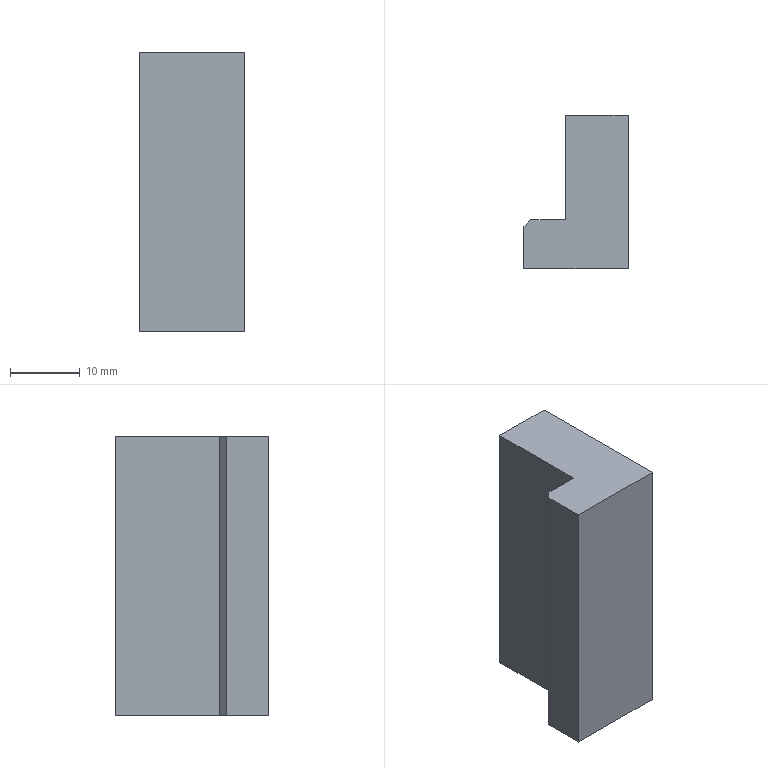Part | STEP file | ASND-0110-Body 1-30 | 1 solid | 9 faces | box 15 x 22 x 40 mm | volume 9580 mm3 | plane 9
STEP:
#1=CARTESIAN_POINT('',(0.,0.,0.));
#2=DIRECTION('',(0.,0.,1.));
#3=DIRECTION('',(1.,0.,0.));
#4=AXIS2_PLACEMENT_3D('',#1,#2,#3);
#5=CARTESIAN_POINT('',(1.,7.,14.));
#6=VERTEX_POINT('',#5);
#7=CARTESIAN_POINT('',(0.,6.,14.));
#8=VERTEX_POINT('',#7);
#9=CARTESIAN_POINT('',(3.,9.,14.));
#10=DIRECTION('',(-0.7071,-0.7071,0.));
#11=VECTOR('',#10,1.);
#12=LINE('',#9,#11);
#13=CARTESIAN_POINT('',(0.5,6.5,27.));
#14=DIRECTION('',(-0.7071,0.7071,0.));
#15=DIRECTION('',(0.5774,0.5774,0.5774));
#16=AXIS2_PLACEMENT_3D('',#13,#14,#15);
#17=PLANE('',#16);
#18=CARTESIAN_POINT('',(-4.619,12.656));
#19=DIRECTION('',(-0.8165,-0.5774));
#20=VECTOR('',#19,1.);
#21=LINE('',#18,#20);
#22=(GEOMETRIC_REPRESENTATION_CONTEXT(2)PARAMETRIC_REPRESENTATION_CONTEXT()REPRESENTATION_CONTEXT('',''));
#23=DEFINITIONAL_REPRESENTATION('',(#21),#22);
#24=PCURVE('',#17,#23);
#25=CARTESIAN_POINT('',(7.5,7.5,14.));
#26=DIRECTION('',(0.,0.,1.));
#27=DIRECTION('',(0.7071,0.7071,0.));
#28=AXIS2_PLACEMENT_3D('',#25,#26,#27);
#29=PLANE('',#28);
#30=CARTESIAN_POINT('',(-2.121,4.243));
#31=DIRECTION('',(-1.,0.));
#32=VECTOR('',#31,1.);
#33=LINE('',#30,#32);
#34=(GEOMETRIC_REPRESENTATION_CONTEXT(2)PARAMETRIC_REPRESENTATION_CONTEXT()REPRESENTATION_CONTEXT('',''));
#35=DEFINITIONAL_REPRESENTATION('',(#33),#34);
#36=PCURVE('',#29,#35);
#37=SURFACE_CURVE('',#12,(#24,#36),.PCURVE_S1.);
#38=EDGE_CURVE('',#6,#8,#37,.T.);
#39=ORIENTED_EDGE('',*,*,#38,.T.);
#40=CARTESIAN_POINT('',(0.,6.,54.));
#41=VERTEX_POINT('',#40);
#42=CARTESIAN_POINT('',(0.,6.,27.));
#43=DIRECTION('',(0.,0.,1.));
#44=VECTOR('',#43,1.);
#45=LINE('',#42,#44);
#46=CARTESIAN_POINT('',(-0.5774,-0.4082));
#47=DIRECTION('',(0.5774,-0.8165));
#48=VECTOR('',#47,1.);
#49=LINE('',#46,#48);
#50=(GEOMETRIC_REPRESENTATION_CONTEXT(2)PARAMETRIC_REPRESENTATION_CONTEXT()REPRESENTATION_CONTEXT('',''));
#51=DEFINITIONAL_REPRESENTATION('',(#49),#50);
#52=PCURVE('',#17,#51);
#53=CARTESIAN_POINT('',(0.,0.,0.));
#54=DIRECTION('',(-1.,0.,0.));
#55=DIRECTION('',(0.,0.7071,0.7071));
#56=AXIS2_PLACEMENT_3D('',#53,#54,#55);
#57=PLANE('',#56);
#58=CARTESIAN_POINT('',(23.335,-14.849));
#59=DIRECTION('',(0.7071,-0.7071));
#60=VECTOR('',#59,1.);
#61=LINE('',#58,#60);
#62=(GEOMETRIC_REPRESENTATION_CONTEXT(2)PARAMETRIC_REPRESENTATION_CONTEXT()REPRESENTATION_CONTEXT('',''));
#63=DEFINITIONAL_REPRESENTATION('',(#61),#62);
#64=PCURVE('',#57,#63);
#65=SURFACE_CURVE('',#45,(#52,#64),.PCURVE_S1.);
#66=EDGE_CURVE('',#8,#41,#65,.T.);
#67=ORIENTED_EDGE('',*,*,#66,.T.);
#68=CARTESIAN_POINT('',(1.,7.,54.));
#69=VERTEX_POINT('',#68);
#70=CARTESIAN_POINT('',(3.,9.,54.));
#71=DIRECTION('',(0.7071,0.7071,0.));
#72=VECTOR('',#71,1.);
#73=LINE('',#70,#72);
#74=CARTESIAN_POINT('',(18.475,-20.004));
#75=DIRECTION('',(0.8165,0.5774));
#76=VECTOR('',#75,1.);
#77=LINE('',#74,#76);
#78=(GEOMETRIC_REPRESENTATION_CONTEXT(2)PARAMETRIC_REPRESENTATION_CONTEXT()REPRESENTATION_CONTEXT('',''));
#79=DEFINITIONAL_REPRESENTATION('',(#77),#78);
#80=PCURVE('',#17,#79);
#81=CARTESIAN_POINT('',(7.5,7.5,54.));
#82=DIRECTION('',(0.,0.,1.));
#83=DIRECTION('',(0.7071,0.7071,0.));
#84=AXIS2_PLACEMENT_3D('',#81,#82,#83);
#85=PLANE('',#84);
#86=CARTESIAN_POINT('',(-2.121,4.243));
#87=DIRECTION('',(1.,0.));
#88=VECTOR('',#87,1.);
#89=LINE('',#86,#88);
#90=(GEOMETRIC_REPRESENTATION_CONTEXT(2)PARAMETRIC_REPRESENTATION_CONTEXT()REPRESENTATION_CONTEXT('',''));
#91=DEFINITIONAL_REPRESENTATION('',(#89),#90);
#92=PCURVE('',#85,#91);
#93=SURFACE_CURVE('',#73,(#80,#92),.PCURVE_S1.);
#94=EDGE_CURVE('',#41,#69,#93,.T.);
#95=ORIENTED_EDGE('',*,*,#94,.T.);
#96=CARTESIAN_POINT('',(1.,7.,27.));
#97=DIRECTION('',(0.,0.,-1.));
#98=VECTOR('',#97,1.);
#99=LINE('',#96,#98);
#100=CARTESIAN_POINT('',(0.5774,0.4082));
#101=DIRECTION('',(-0.5774,0.8165));
#102=VECTOR('',#101,1.);
#103=LINE('',#100,#102);
#104=(GEOMETRIC_REPRESENTATION_CONTEXT(2)PARAMETRIC_REPRESENTATION_CONTEXT()REPRESENTATION_CONTEXT('',''));
#105=DEFINITIONAL_REPRESENTATION('',(#103),#104);
#106=PCURVE('',#17,#105);
#107=CARTESIAN_POINT('',(0.,7.,54.));
#108=DIRECTION('',(0.,-1.,0.));
#109=DIRECTION('',(0.7071,0.,0.7071));
#110=AXIS2_PLACEMENT_3D('',#107,#108,#109);
#111=PLANE('',#110);
#112=CARTESIAN_POINT('',(-18.385,-19.799));
#113=DIRECTION('',(-0.7071,-0.7071));
#114=VECTOR('',#113,1.);
#115=LINE('',#112,#114);
#116=(GEOMETRIC_REPRESENTATION_CONTEXT(2)PARAMETRIC_REPRESENTATION_CONTEXT()REPRESENTATION_CONTEXT('',''));
#117=DEFINITIONAL_REPRESENTATION('',(#115),#116);
#118=PCURVE('',#111,#117);
#119=SURFACE_CURVE('',#99,(#106,#118),.PCURVE_S1.);
#120=EDGE_CURVE('',#69,#6,#119,.T.);
#121=ORIENTED_EDGE('',*,*,#120,.T.);
#122=EDGE_LOOP('',(#39,#67,#95,#121));
#123=FACE_BOUND('',#122,.T.);
#124=ADVANCED_FACE('',(#123),#17,.T.);
#125=ORIENTED_EDGE('',*,*,#38,.F.);
#126=CARTESIAN_POINT('',(6.,7.,14.));
#127=VERTEX_POINT('',#126);
#128=CARTESIAN_POINT('',(3.75,7.,14.));
#129=DIRECTION('',(1.,0.,0.));
#130=VECTOR('',#129,1.);
#131=LINE('',#128,#130);
#132=CARTESIAN_POINT('',(-3.005,2.298));
#133=DIRECTION('',(0.7071,-0.7071));
#134=VECTOR('',#133,1.);
#135=LINE('',#132,#134);
#136=(GEOMETRIC_REPRESENTATION_CONTEXT(2)PARAMETRIC_REPRESENTATION_CONTEXT()REPRESENTATION_CONTEXT('',''));
#137=DEFINITIONAL_REPRESENTATION('',(#135),#136);
#138=PCURVE('',#29,#137);
#139=CARTESIAN_POINT('',(-25.633,-30.936));
#140=DIRECTION('',(0.7071,-0.7071));
#141=VECTOR('',#140,1.);
#142=LINE('',#139,#141);
#143=(GEOMETRIC_REPRESENTATION_CONTEXT(2)PARAMETRIC_REPRESENTATION_CONTEXT()REPRESENTATION_CONTEXT('',''));
#144=DEFINITIONAL_REPRESENTATION('',(#142),#143);
#145=PCURVE('',#111,#144);
#146=SURFACE_CURVE('',#131,(#138,#145),.PCURVE_S1.);
#147=EDGE_CURVE('',#6,#127,#146,.T.);
#148=ORIENTED_EDGE('',*,*,#147,.T.);
#149=CARTESIAN_POINT('',(6.,22.,14.));
#150=VERTEX_POINT('',#149);
#151=CARTESIAN_POINT('',(6.,6.25,14.));
#152=DIRECTION('',(0.,1.,0.));
#153=VECTOR('',#152,1.);
#154=LINE('',#151,#153);
#155=CARTESIAN_POINT('',(-1.945,0.1768));
#156=DIRECTION('',(0.7071,0.7071));
#157=VECTOR('',#156,1.);
#158=LINE('',#155,#157);
#159=(GEOMETRIC_REPRESENTATION_CONTEXT(2)PARAMETRIC_REPRESENTATION_CONTEXT()REPRESENTATION_CONTEXT('',''));
#160=DEFINITIONAL_REPRESENTATION('',(#158),#159);
#161=PCURVE('',#29,#160);
#162=CARTESIAN_POINT('',(6.,5.,54.));
#163=DIRECTION('',(1.,0.,0.));
#164=DIRECTION('',(0.,0.7071,0.7071));
#165=AXIS2_PLACEMENT_3D('',#162,#163,#164);
#166=PLANE('',#165);
#167=CARTESIAN_POINT('',(-27.4,-29.168));
#168=DIRECTION('',(0.7071,-0.7071));
#169=VECTOR('',#168,1.);
#170=LINE('',#167,#169);
#171=(GEOMETRIC_REPRESENTATION_CONTEXT(2)PARAMETRIC_REPRESENTATION_CONTEXT()REPRESENTATION_CONTEXT('',''));
#172=DEFINITIONAL_REPRESENTATION('',(#170),#171);
#173=PCURVE('',#166,#172);
#174=SURFACE_CURVE('',#154,(#161,#173),.PCURVE_S1.);
#175=EDGE_CURVE('',#127,#150,#174,.T.);
#176=ORIENTED_EDGE('',*,*,#175,.T.);
#177=CARTESIAN_POINT('',(15.,22.,14.));
#178=VERTEX_POINT('',#177);
#179=CARTESIAN_POINT('',(15.,22.,14.));
#180=DIRECTION('',(-1.,0.,0.));
#181=VECTOR('',#180,1.);
#182=LINE('',#179,#181);
#183=CARTESIAN_POINT('',(15.556,4.95));
#184=DIRECTION('',(-0.7071,0.7071));
#185=VECTOR('',#184,1.);
#186=LINE('',#183,#185);
#187=(GEOMETRIC_REPRESENTATION_CONTEXT(2)PARAMETRIC_REPRESENTATION_CONTEXT()REPRESENTATION_CONTEXT('',''));
#188=DEFINITIONAL_REPRESENTATION('',(#186),#187);
#189=PCURVE('',#29,#188);
#190=CARTESIAN_POINT('',(0.,22.,0.));
#191=DIRECTION('',(0.,1.,0.));
#192=DIRECTION('',(0.7071,0.,0.7071));
#193=AXIS2_PLACEMENT_3D('',#190,#191,#192);
#194=PLANE('',#193);
#195=CARTESIAN_POINT('',(20.506,0.7071));
#196=DIRECTION('',(-0.7071,-0.7071));
#197=VECTOR('',#196,1.);
#198=LINE('',#195,#197);
#199=(GEOMETRIC_REPRESENTATION_CONTEXT(2)PARAMETRIC_REPRESENTATION_CONTEXT()REPRESENTATION_CONTEXT('',''));
#200=DEFINITIONAL_REPRESENTATION('',(#198),#199);
#201=PCURVE('',#194,#200);
#202=SURFACE_CURVE('',#182,(#189,#201),.PCURVE_S1.);
#203=EDGE_CURVE('',#178,#150,#202,.T.);
#204=ORIENTED_EDGE('',*,*,#203,.F.);
#205=CARTESIAN_POINT('',(15.,0.,14.));
#206=VERTEX_POINT('',#205);
#207=CARTESIAN_POINT('',(15.,0.,14.));
#208=DIRECTION('',(0.,1.,0.));
#209=VECTOR('',#208,1.);
#210=LINE('',#207,#209);
#211=CARTESIAN_POINT('',(0.,-10.607));
#212=DIRECTION('',(0.7071,0.7071));
#213=VECTOR('',#212,1.);
#214=LINE('',#211,#213);
#215=(GEOMETRIC_REPRESENTATION_CONTEXT(2)PARAMETRIC_REPRESENTATION_CONTEXT()REPRESENTATION_CONTEXT('',''));
#216=DEFINITIONAL_REPRESENTATION('',(#214),#215);
#217=PCURVE('',#29,#216);
#218=CARTESIAN_POINT('',(15.,15.,0.));
#219=DIRECTION('',(1.,0.,0.));
#220=DIRECTION('',(0.,0.7071,0.7071));
#221=AXIS2_PLACEMENT_3D('',#218,#219,#220);
#222=PLANE('',#221);
#223=CARTESIAN_POINT('',(-0.7071,20.506));
#224=DIRECTION('',(0.7071,-0.7071));
#225=VECTOR('',#224,1.);
#226=LINE('',#223,#225);
#227=(GEOMETRIC_REPRESENTATION_CONTEXT(2)PARAMETRIC_REPRESENTATION_CONTEXT()REPRESENTATION_CONTEXT('',''));
#228=DEFINITIONAL_REPRESENTATION('',(#226),#227);
#229=PCURVE('',#222,#228);
#230=SURFACE_CURVE('',#210,(#217,#229),.PCURVE_S1.);
#231=EDGE_CURVE('',#206,#178,#230,.T.);
#232=ORIENTED_EDGE('',*,*,#231,.F.);
#233=CARTESIAN_POINT('',(0.,0.,14.));
#234=VERTEX_POINT('',#233);
#235=CARTESIAN_POINT('',(0.,0.,14.));
#236=DIRECTION('',(1.,0.,0.));
#237=VECTOR('',#236,1.);
#238=LINE('',#235,#237);
#239=CARTESIAN_POINT('',(-10.607,0.));
#240=DIRECTION('',(0.7071,-0.7071));
#241=VECTOR('',#240,1.);
#242=LINE('',#239,#241);
#243=(GEOMETRIC_REPRESENTATION_CONTEXT(2)PARAMETRIC_REPRESENTATION_CONTEXT()REPRESENTATION_CONTEXT('',''));
#244=DEFINITIONAL_REPRESENTATION('',(#242),#243);
#245=PCURVE('',#29,#244);
#246=CARTESIAN_POINT('',(15.,0.,0.));
#247=DIRECTION('',(0.,-1.,0.));
#248=DIRECTION('',(0.7071,0.,0.7071));
#249=AXIS2_PLACEMENT_3D('',#246,#247,#248);
#250=PLANE('',#249);
#251=CARTESIAN_POINT('',(-0.7071,20.506));
#252=DIRECTION('',(0.7071,-0.7071));
#253=VECTOR('',#252,1.);
#254=LINE('',#251,#253);
#255=(GEOMETRIC_REPRESENTATION_CONTEXT(2)PARAMETRIC_REPRESENTATION_CONTEXT()REPRESENTATION_CONTEXT('',''));
#256=DEFINITIONAL_REPRESENTATION('',(#254),#255);
#257=PCURVE('',#250,#256);
#258=SURFACE_CURVE('',#238,(#245,#257),.PCURVE_S1.);
#259=EDGE_CURVE('',#234,#206,#258,.T.);
#260=ORIENTED_EDGE('',*,*,#259,.F.);
#261=CARTESIAN_POINT('',(0.,15.,14.));
#262=DIRECTION('',(0.,-1.,0.));
#263=VECTOR('',#262,1.);
#264=LINE('',#261,#263);
#265=CARTESIAN_POINT('',(0.,10.607));
#266=DIRECTION('',(-0.7071,-0.7071));
#267=VECTOR('',#266,1.);
#268=LINE('',#265,#267);
#269=(GEOMETRIC_REPRESENTATION_CONTEXT(2)PARAMETRIC_REPRESENTATION_CONTEXT()REPRESENTATION_CONTEXT('',''));
#270=DEFINITIONAL_REPRESENTATION('',(#268),#269);
#271=PCURVE('',#29,#270);
#272=CARTESIAN_POINT('',(20.506,0.7071));
#273=DIRECTION('',(-0.7071,-0.7071));
#274=VECTOR('',#273,1.);
#275=LINE('',#272,#274);
#276=(GEOMETRIC_REPRESENTATION_CONTEXT(2)PARAMETRIC_REPRESENTATION_CONTEXT()REPRESENTATION_CONTEXT('',''));
#277=DEFINITIONAL_REPRESENTATION('',(#275),#276);
#278=PCURVE('',#57,#277);
#279=SURFACE_CURVE('',#264,(#271,#278),.PCURVE_S1.);
#280=EDGE_CURVE('',#8,#234,#279,.T.);
#281=ORIENTED_EDGE('',*,*,#280,.F.);
#282=EDGE_LOOP('',(#125,#148,#176,#204,#232,#260,#281));
#283=FACE_BOUND('',#282,.T.);
#284=ADVANCED_FACE('',(#283),#29,.F.);
#285=ORIENTED_EDGE('',*,*,#120,.F.);
#286=CARTESIAN_POINT('',(6.,7.,54.));
#287=VERTEX_POINT('',#286);
#288=CARTESIAN_POINT('',(3.75,7.,54.));
#289=DIRECTION('',(-1.,0.,0.));
#290=VECTOR('',#289,1.);
#291=LINE('',#288,#290);
#292=CARTESIAN_POINT('',(2.652,-2.652));
#293=DIRECTION('',(-0.7071,0.7071));
#294=VECTOR('',#293,1.);
#295=LINE('',#292,#294);
#296=(GEOMETRIC_REPRESENTATION_CONTEXT(2)PARAMETRIC_REPRESENTATION_CONTEXT()REPRESENTATION_CONTEXT('',''));
#297=DEFINITIONAL_REPRESENTATION('',(#295),#296);
#298=PCURVE('',#111,#297);
#299=CARTESIAN_POINT('',(-3.005,2.298));
#300=DIRECTION('',(-0.7071,0.7071));
#301=VECTOR('',#300,1.);
#302=LINE('',#299,#301);
#303=(GEOMETRIC_REPRESENTATION_CONTEXT(2)PARAMETRIC_REPRESENTATION_CONTEXT()REPRESENTATION_CONTEXT('',''));
#304=DEFINITIONAL_REPRESENTATION('',(#302),#303);
#305=PCURVE('',#85,#304);
#306=SURFACE_CURVE('',#291,(#298,#305),.PCURVE_S1.);
#307=EDGE_CURVE('',#287,#69,#306,.T.);
#308=ORIENTED_EDGE('',*,*,#307,.F.);
#309=CARTESIAN_POINT('',(6.,7.,54.));
#310=DIRECTION('',(0.,0.,-1.));
#311=VECTOR('',#310,1.);
#312=LINE('',#309,#311);
#313=CARTESIAN_POINT('',(4.243,-4.243));
#314=DIRECTION('',(-0.7071,-0.7071));
#315=VECTOR('',#314,1.);
#316=LINE('',#313,#315);
#317=(GEOMETRIC_REPRESENTATION_CONTEXT(2)PARAMETRIC_REPRESENTATION_CONTEXT()REPRESENTATION_CONTEXT('',''));
#318=DEFINITIONAL_REPRESENTATION('',(#316),#317);
#319=PCURVE('',#111,#318);
#320=CARTESIAN_POINT('',(1.414,-1.414));
#321=DIRECTION('',(-0.7071,-0.7071));
#322=VECTOR('',#321,1.);
#323=LINE('',#320,#322);
#324=(GEOMETRIC_REPRESENTATION_CONTEXT(2)PARAMETRIC_REPRESENTATION_CONTEXT()REPRESENTATION_CONTEXT('',''));
#325=DEFINITIONAL_REPRESENTATION('',(#323),#324);
#326=PCURVE('',#166,#325);
#327=SURFACE_CURVE('',#312,(#319,#326),.PCURVE_S1.);
#328=EDGE_CURVE('',#287,#127,#327,.T.);
#329=ORIENTED_EDGE('',*,*,#328,.T.);
#330=ORIENTED_EDGE('',*,*,#147,.F.);
#331=EDGE_LOOP('',(#285,#308,#329,#330));
#332=FACE_BOUND('',#331,.T.);
#333=ADVANCED_FACE('',(#332),#111,.F.);
#334=ORIENTED_EDGE('',*,*,#175,.F.);
#335=ORIENTED_EDGE('',*,*,#328,.F.);
#336=CARTESIAN_POINT('',(6.,22.,54.));
#337=VERTEX_POINT('',#336);
#338=CARTESIAN_POINT('',(6.,6.25,54.));
#339=DIRECTION('',(0.,-1.,0.));
#340=VECTOR('',#339,1.);
#341=LINE('',#338,#340);
#342=CARTESIAN_POINT('',(0.8839,-0.8839));
#343=DIRECTION('',(-0.7071,0.7071));
#344=VECTOR('',#343,1.);
#345=LINE('',#342,#344);
#346=(GEOMETRIC_REPRESENTATION_CONTEXT(2)PARAMETRIC_REPRESENTATION_CONTEXT()REPRESENTATION_CONTEXT('',''));
#347=DEFINITIONAL_REPRESENTATION('',(#345),#346);
#348=PCURVE('',#166,#347);
#349=CARTESIAN_POINT('',(-1.945,0.1768));
#350=DIRECTION('',(-0.7071,-0.7071));
#351=VECTOR('',#350,1.);
#352=LINE('',#349,#351);
#353=(GEOMETRIC_REPRESENTATION_CONTEXT(2)PARAMETRIC_REPRESENTATION_CONTEXT()REPRESENTATION_CONTEXT('',''));
#354=DEFINITIONAL_REPRESENTATION('',(#352),#353);
#355=PCURVE('',#85,#354);
#356=SURFACE_CURVE('',#341,(#348,#355),.PCURVE_S1.);
#357=EDGE_CURVE('',#337,#287,#356,.T.);
#358=ORIENTED_EDGE('',*,*,#357,.F.);
#359=CARTESIAN_POINT('',(6.,22.,27.));
#360=DIRECTION('',(0.,0.,1.));
#361=VECTOR('',#360,1.);
#362=LINE('',#359,#361);
#363=CARTESIAN_POINT('',(-7.071,-31.113));
#364=DIRECTION('',(0.7071,0.7071));
#365=VECTOR('',#364,1.);
#366=LINE('',#363,#365);
#367=(GEOMETRIC_REPRESENTATION_CONTEXT(2)PARAMETRIC_REPRESENTATION_CONTEXT()REPRESENTATION_CONTEXT('',''));
#368=DEFINITIONAL_REPRESENTATION('',(#366),#367);
#369=PCURVE('',#166,#368);
#370=CARTESIAN_POINT('',(23.335,-14.849));
#371=DIRECTION('',(0.7071,-0.7071));
#372=VECTOR('',#371,1.);
#373=LINE('',#370,#372);
#374=(GEOMETRIC_REPRESENTATION_CONTEXT(2)PARAMETRIC_REPRESENTATION_CONTEXT()REPRESENTATION_CONTEXT('',''));
#375=DEFINITIONAL_REPRESENTATION('',(#373),#374);
#376=PCURVE('',#194,#375);
#377=SURFACE_CURVE('',#362,(#369,#376),.PCURVE_S1.);
#378=EDGE_CURVE('',#150,#337,#377,.T.);
#379=ORIENTED_EDGE('',*,*,#378,.F.);
#380=EDGE_LOOP('',(#334,#335,#358,#379));
#381=FACE_BOUND('',#380,.T.);
#382=ADVANCED_FACE('',(#381),#166,.F.);
#383=ORIENTED_EDGE('',*,*,#94,.F.);
#384=CARTESIAN_POINT('',(0.,0.,54.));
#385=VERTEX_POINT('',#384);
#386=CARTESIAN_POINT('',(0.,15.,54.));
#387=DIRECTION('',(0.,1.,0.));
#388=VECTOR('',#387,1.);
#389=LINE('',#386,#388);
#390=CARTESIAN_POINT('',(0.,10.607));
#391=DIRECTION('',(0.7071,0.7071));
#392=VECTOR('',#391,1.);
#393=LINE('',#390,#392);
#394=(GEOMETRIC_REPRESENTATION_CONTEXT(2)PARAMETRIC_REPRESENTATION_CONTEXT()REPRESENTATION_CONTEXT('',''));
#395=DEFINITIONAL_REPRESENTATION('',(#393),#394);
#396=PCURVE('',#85,#395);
#397=CARTESIAN_POINT('',(48.79,-27.577));
#398=DIRECTION('',(0.7071,0.7071));
#399=VECTOR('',#398,1.);
#400=LINE('',#397,#399);
#401=(GEOMETRIC_REPRESENTATION_CONTEXT(2)PARAMETRIC_REPRESENTATION_CONTEXT()REPRESENTATION_CONTEXT('',''));
#402=DEFINITIONAL_REPRESENTATION('',(#400),#401);
#403=PCURVE('',#57,#402);
#404=SURFACE_CURVE('',#389,(#396,#403),.PCURVE_S1.);
#405=EDGE_CURVE('',#385,#41,#404,.T.);
#406=ORIENTED_EDGE('',*,*,#405,.F.);
#407=CARTESIAN_POINT('',(15.,0.,54.));
#408=VERTEX_POINT('',#407);
#409=CARTESIAN_POINT('',(0.,0.,54.));
#410=DIRECTION('',(-1.,0.,0.));
#411=VECTOR('',#410,1.);
#412=LINE('',#409,#411);
#413=CARTESIAN_POINT('',(-10.607,0.));
#414=DIRECTION('',(-0.7071,0.7071));
#415=VECTOR('',#414,1.);
#416=LINE('',#413,#415);
#417=(GEOMETRIC_REPRESENTATION_CONTEXT(2)PARAMETRIC_REPRESENTATION_CONTEXT()REPRESENTATION_CONTEXT('',''));
#418=DEFINITIONAL_REPRESENTATION('',(#416),#417);
#419=PCURVE('',#85,#418);
#420=CARTESIAN_POINT('',(27.577,48.79));
#421=DIRECTION('',(-0.7071,0.7071));
#422=VECTOR('',#421,1.);
#423=LINE('',#420,#422);
#424=(GEOMETRIC_REPRESENTATION_CONTEXT(2)PARAMETRIC_REPRESENTATION_CONTEXT()REPRESENTATION_CONTEXT('',''));
#425=DEFINITIONAL_REPRESENTATION('',(#423),#424);
#426=PCURVE('',#250,#425);
#427=SURFACE_CURVE('',#412,(#419,#426),.PCURVE_S1.);
#428=EDGE_CURVE('',#408,#385,#427,.T.);
#429=ORIENTED_EDGE('',*,*,#428,.F.);
#430=CARTESIAN_POINT('',(15.,22.,54.));
#431=VERTEX_POINT('',#430);
#432=CARTESIAN_POINT('',(15.,0.,54.));
#433=DIRECTION('',(0.,-1.,0.));
#434=VECTOR('',#433,1.);
#435=LINE('',#432,#434);
#436=CARTESIAN_POINT('',(0.,-10.607));
#437=DIRECTION('',(-0.7071,-0.7071));
#438=VECTOR('',#437,1.);
#439=LINE('',#436,#438);
#440=(GEOMETRIC_REPRESENTATION_CONTEXT(2)PARAMETRIC_REPRESENTATION_CONTEXT()REPRESENTATION_CONTEXT('',''));
#441=DEFINITIONAL_REPRESENTATION('',(#439),#440);
#442=PCURVE('',#85,#441);
#443=CARTESIAN_POINT('',(27.577,48.79));
#444=DIRECTION('',(-0.7071,0.7071));
#445=VECTOR('',#444,1.);
#446=LINE('',#443,#445);
#447=(GEOMETRIC_REPRESENTATION_CONTEXT(2)PARAMETRIC_REPRESENTATION_CONTEXT()REPRESENTATION_CONTEXT('',''));
#448=DEFINITIONAL_REPRESENTATION('',(#446),#447);
#449=PCURVE('',#222,#448);
#450=SURFACE_CURVE('',#435,(#442,#449),.PCURVE_S1.);
#451=EDGE_CURVE('',#431,#408,#450,.T.);
#452=ORIENTED_EDGE('',*,*,#451,.F.);
#453=CARTESIAN_POINT('',(15.,22.,54.));
#454=DIRECTION('',(1.,0.,0.));
#455=VECTOR('',#454,1.);
#456=LINE('',#453,#455);
#457=CARTESIAN_POINT('',(15.556,4.95));
#458=DIRECTION('',(0.7071,-0.7071));
#459=VECTOR('',#458,1.);
#460=LINE('',#457,#459);
#461=(GEOMETRIC_REPRESENTATION_CONTEXT(2)PARAMETRIC_REPRESENTATION_CONTEXT()REPRESENTATION_CONTEXT('',''));
#462=DEFINITIONAL_REPRESENTATION('',(#460),#461);
#463=PCURVE('',#85,#462);
#464=CARTESIAN_POINT('',(48.79,-27.577));
#465=DIRECTION('',(0.7071,0.7071));
#466=VECTOR('',#465,1.);
#467=LINE('',#464,#466);
#468=(GEOMETRIC_REPRESENTATION_CONTEXT(2)PARAMETRIC_REPRESENTATION_CONTEXT()REPRESENTATION_CONTEXT('',''));
#469=DEFINITIONAL_REPRESENTATION('',(#467),#468);
#470=PCURVE('',#194,#469);
#471=SURFACE_CURVE('',#456,(#463,#470),.PCURVE_S1.);
#472=EDGE_CURVE('',#337,#431,#471,.T.);
#473=ORIENTED_EDGE('',*,*,#472,.F.);
#474=ORIENTED_EDGE('',*,*,#357,.T.);
#475=ORIENTED_EDGE('',*,*,#307,.T.);
#476=EDGE_LOOP('',(#383,#406,#429,#452,#473,#474,#475));
#477=FACE_BOUND('',#476,.T.);
#478=ADVANCED_FACE('',(#477),#85,.T.);
#479=ORIENTED_EDGE('',*,*,#66,.F.);
#480=ORIENTED_EDGE('',*,*,#280,.T.);
#481=CARTESIAN_POINT('',(0.,0.,0.));
#482=DIRECTION('',(0.,0.,1.));
#483=VECTOR('',#482,1.);
#484=LINE('',#481,#483);
#485=CARTESIAN_POINT('',(0.,0.));
#486=DIRECTION('',(0.7071,-0.7071));
#487=VECTOR('',#486,1.);
#488=LINE('',#485,#487);
#489=(GEOMETRIC_REPRESENTATION_CONTEXT(2)PARAMETRIC_REPRESENTATION_CONTEXT()REPRESENTATION_CONTEXT('',''));
#490=DEFINITIONAL_REPRESENTATION('',(#488),#489);
#491=PCURVE('',#57,#490);
#492=CARTESIAN_POINT('',(-10.607,10.607));
#493=DIRECTION('',(0.7071,0.7071));
#494=VECTOR('',#493,1.);
#495=LINE('',#492,#494);
#496=(GEOMETRIC_REPRESENTATION_CONTEXT(2)PARAMETRIC_REPRESENTATION_CONTEXT()REPRESENTATION_CONTEXT('',''));
#497=DEFINITIONAL_REPRESENTATION('',(#495),#496);
#498=PCURVE('',#250,#497);
#499=SURFACE_CURVE('',#484,(#491,#498),.PCURVE_S1.);
#500=EDGE_CURVE('',#234,#385,#499,.T.);
#501=ORIENTED_EDGE('',*,*,#500,.T.);
#502=ORIENTED_EDGE('',*,*,#405,.T.);
#503=EDGE_LOOP('',(#479,#480,#501,#502));
#504=FACE_BOUND('',#503,.T.);
#505=ADVANCED_FACE('',(#504),#57,.T.);
#506=ORIENTED_EDGE('',*,*,#378,.T.);
#507=ORIENTED_EDGE('',*,*,#472,.T.);
#508=CARTESIAN_POINT('',(15.,22.,0.));
#509=DIRECTION('',(0.,0.,1.));
#510=VECTOR('',#509,1.);
#511=LINE('',#508,#510);
#512=CARTESIAN_POINT('',(10.607,10.607));
#513=DIRECTION('',(0.7071,-0.7071));
#514=VECTOR('',#513,1.);
#515=LINE('',#512,#514);
#516=(GEOMETRIC_REPRESENTATION_CONTEXT(2)PARAMETRIC_REPRESENTATION_CONTEXT()REPRESENTATION_CONTEXT('',''));
#517=DEFINITIONAL_REPRESENTATION('',(#515),#516);
#518=PCURVE('',#194,#517);
#519=CARTESIAN_POINT('',(4.95,-4.95));
#520=DIRECTION('',(0.7071,0.7071));
#521=VECTOR('',#520,1.);
#522=LINE('',#519,#521);
#523=(GEOMETRIC_REPRESENTATION_CONTEXT(2)PARAMETRIC_REPRESENTATION_CONTEXT()REPRESENTATION_CONTEXT('',''));
#524=DEFINITIONAL_REPRESENTATION('',(#522),#523);
#525=PCURVE('',#222,#524);
#526=SURFACE_CURVE('',#511,(#518,#525),.PCURVE_S1.);
#527=EDGE_CURVE('',#178,#431,#526,.T.);
#528=ORIENTED_EDGE('',*,*,#527,.F.);
#529=ORIENTED_EDGE('',*,*,#203,.T.);
#530=EDGE_LOOP('',(#506,#507,#528,#529));
#531=FACE_BOUND('',#530,.T.);
#532=ADVANCED_FACE('',(#531),#194,.T.);
#533=ORIENTED_EDGE('',*,*,#451,.T.);
#534=CARTESIAN_POINT('',(15.,0.,0.));
#535=DIRECTION('',(0.,0.,1.));
#536=VECTOR('',#535,1.);
#537=LINE('',#534,#536);
#538=CARTESIAN_POINT('',(-10.607,10.607));
#539=DIRECTION('',(0.7071,0.7071));
#540=VECTOR('',#539,1.);
#541=LINE('',#538,#540);
#542=(GEOMETRIC_REPRESENTATION_CONTEXT(2)PARAMETRIC_REPRESENTATION_CONTEXT()REPRESENTATION_CONTEXT('',''));
#543=DEFINITIONAL_REPRESENTATION('',(#541),#542);
#544=PCURVE('',#222,#543);
#545=CARTESIAN_POINT('',(0.,0.));
#546=DIRECTION('',(0.7071,0.7071));
#547=VECTOR('',#546,1.);
#548=LINE('',#545,#547);
#549=(GEOMETRIC_REPRESENTATION_CONTEXT(2)PARAMETRIC_REPRESENTATION_CONTEXT()REPRESENTATION_CONTEXT('',''));
#550=DEFINITIONAL_REPRESENTATION('',(#548),#549);
#551=PCURVE('',#250,#550);
#552=SURFACE_CURVE('',#537,(#544,#551),.PCURVE_S1.);
#553=EDGE_CURVE('',#206,#408,#552,.T.);
#554=ORIENTED_EDGE('',*,*,#553,.F.);
#555=ORIENTED_EDGE('',*,*,#231,.T.);
#556=ORIENTED_EDGE('',*,*,#527,.T.);
#557=EDGE_LOOP('',(#533,#554,#555,#556));
#558=FACE_BOUND('',#557,.T.);
#559=ADVANCED_FACE('',(#558),#222,.T.);
#560=ORIENTED_EDGE('',*,*,#428,.T.);
#561=ORIENTED_EDGE('',*,*,#500,.F.);
#562=ORIENTED_EDGE('',*,*,#259,.T.);
#563=ORIENTED_EDGE('',*,*,#553,.T.);
#564=EDGE_LOOP('',(#560,#561,#562,#563));
#565=FACE_BOUND('',#564,.T.);
#566=ADVANCED_FACE('',(#565),#250,.T.);
#567=CLOSED_SHELL('',(#124,#284,#333,#382,#478,#505,#532,#559,#566));
#568=MANIFOLD_SOLID_BREP('',#567);
#569=(LENGTH_UNIT()NAMED_UNIT(*)SI_UNIT(.MILLI.,.METRE.));
#570=UNCERTAINTY_MEASURE_WITH_UNIT(LENGTH_MEASURE(0.0000001),#569,'','');
#571=(NAMED_UNIT(*)PLANE_ANGLE_UNIT()SI_UNIT($,.RADIAN.));
#572=(NAMED_UNIT(*)SI_UNIT($,.STERADIAN.)SOLID_ANGLE_UNIT());
#573=(GEOMETRIC_REPRESENTATION_CONTEXT(3)GLOBAL_UNCERTAINTY_ASSIGNED_CONTEXT((#570))GLOBAL_UNIT_ASSIGNED_CONTEXT((#569,#571,#572))REPRESENTATION_CONTEXT('',''));
#574=ADVANCED_BREP_SHAPE_REPRESENTATION('',(#4,#568),#573);